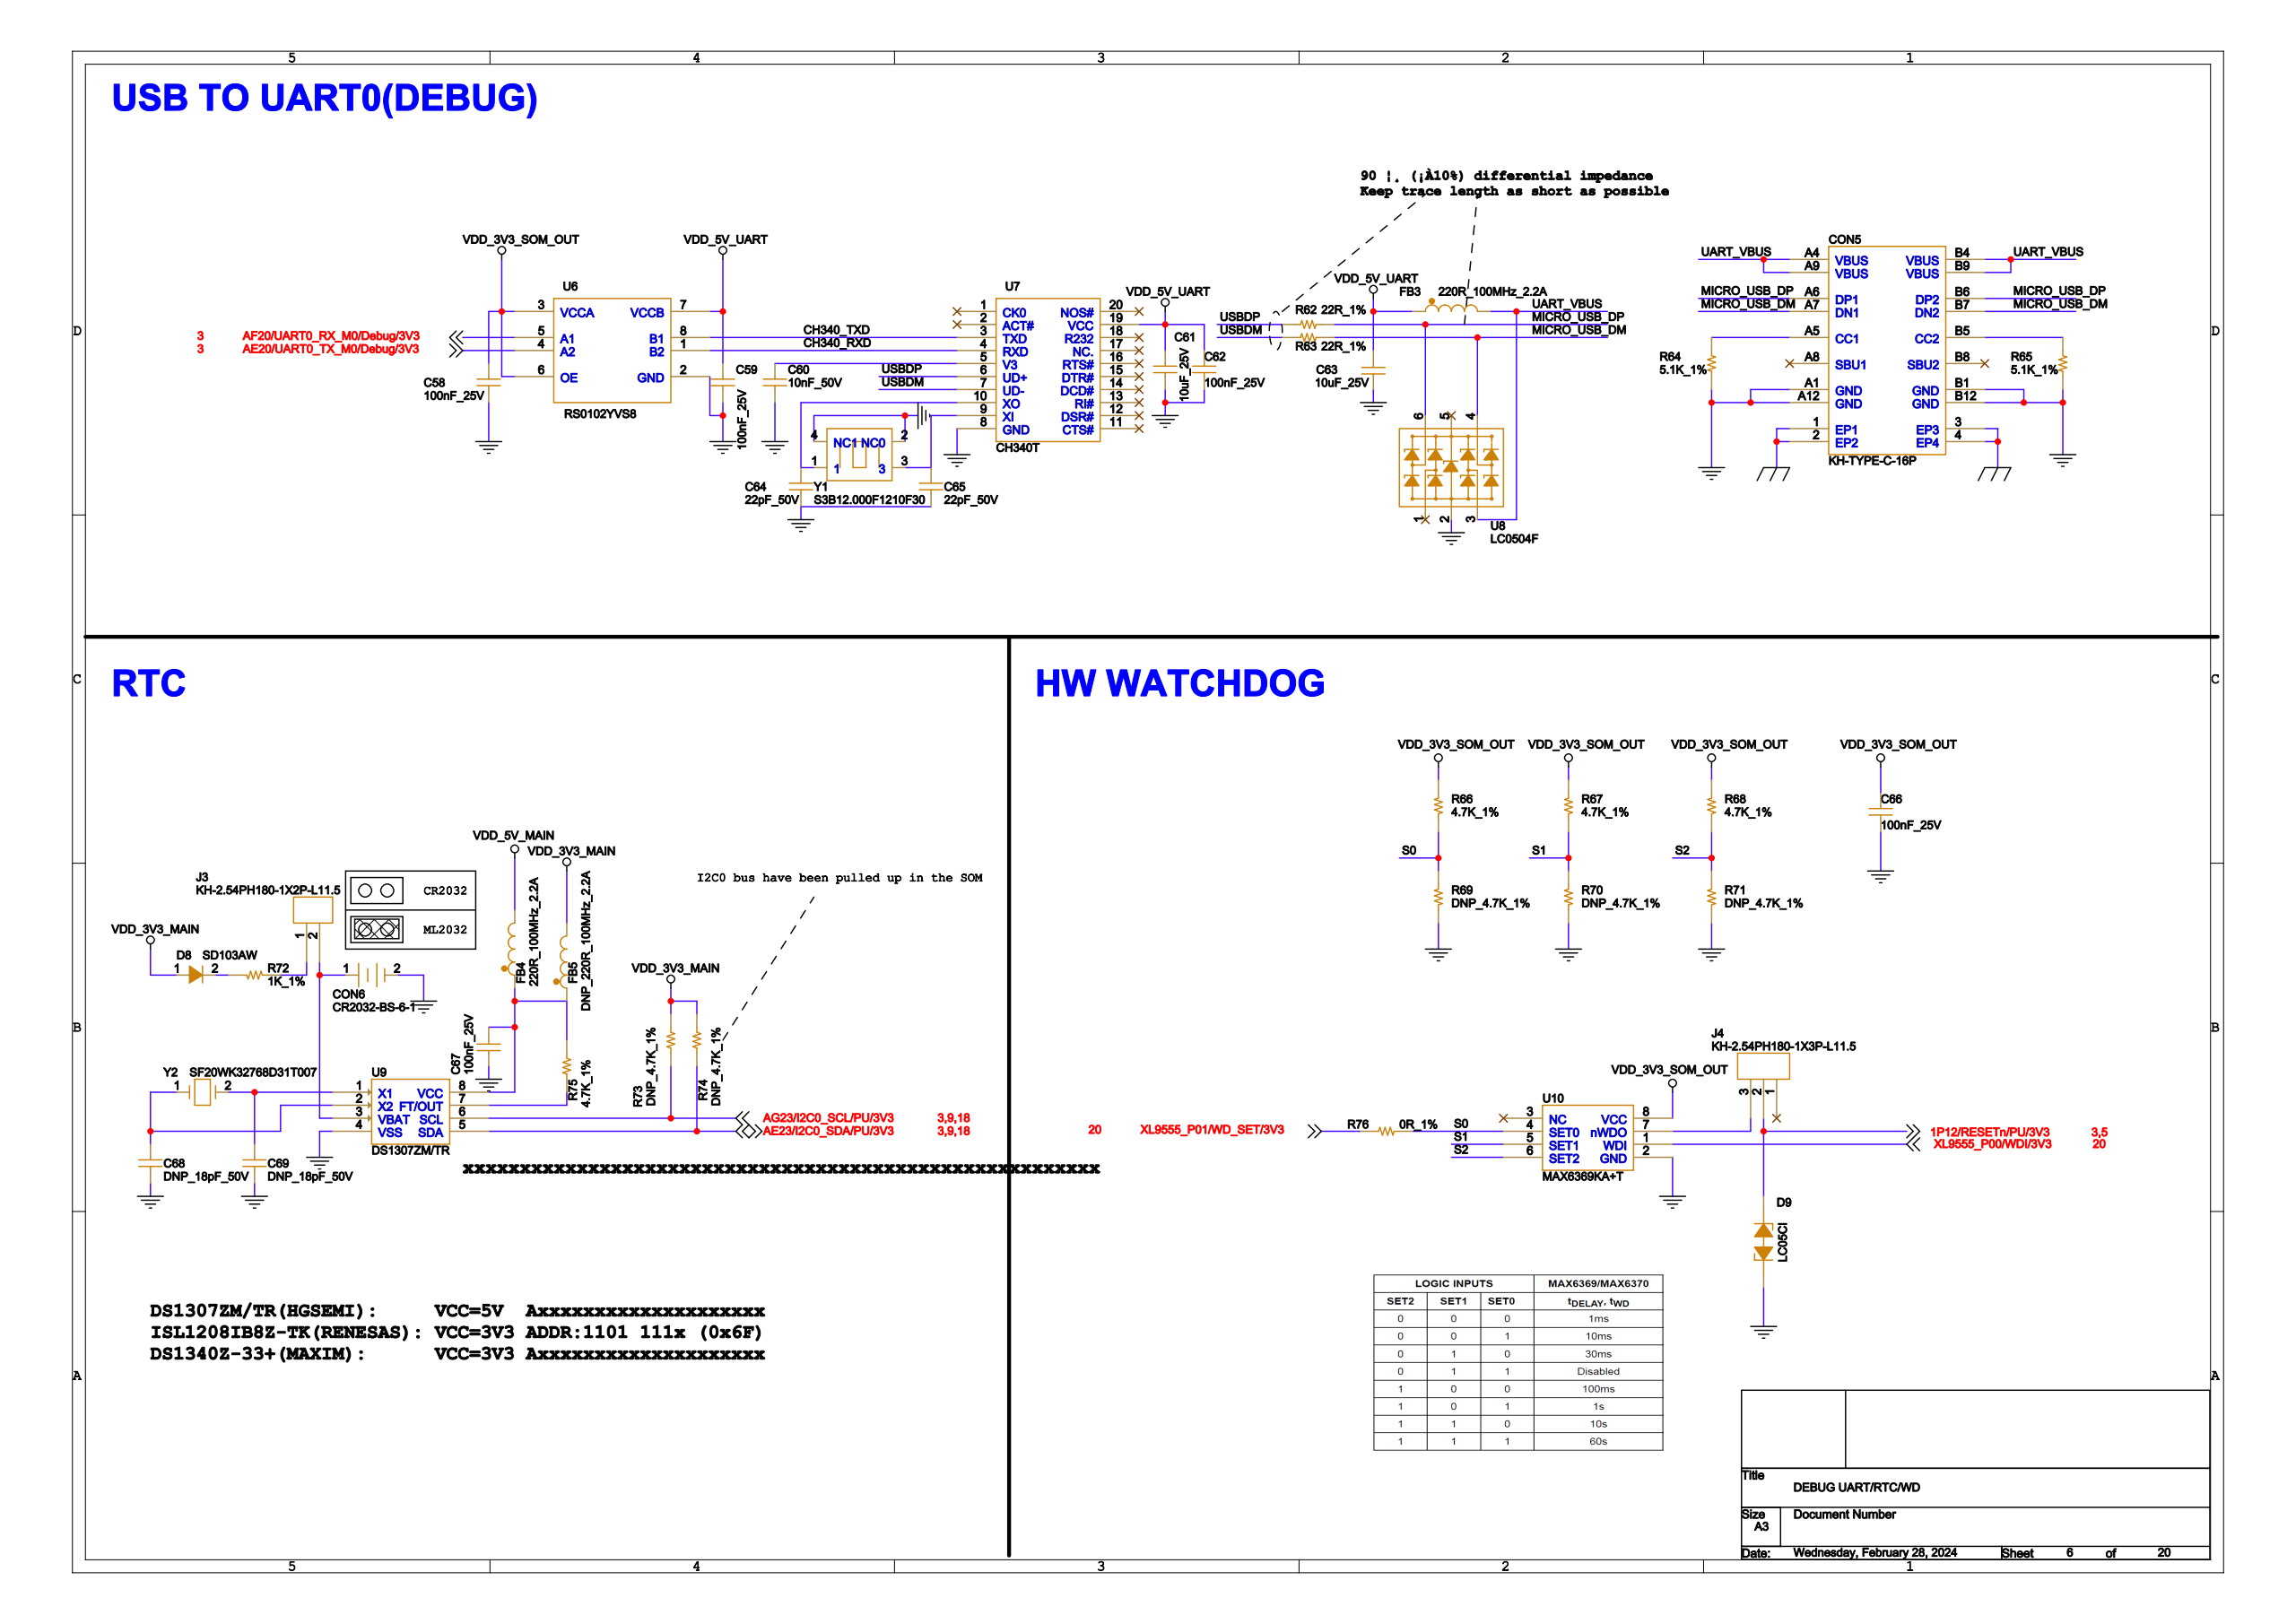Circuit board | Cadence Allegro | 1024 parts | 682 nets | one sheet of the schematic
Parts on this sheet (reference | value | footprint):
C58 | 100nF_25V | C0402
C60 | 10nF_50V | C0402
C62 | 100nF_25V | C0402
C63 | 10uF_25V | C0603
C64 | 22pF_50V | C0603
C65 | 22pF_50V | C0603
C66 | 100nF_25V | C0402
C67 | 100nF_25V | C0402
C68 | DNP_18pF_50V | C0603
C69 | DNP_18pF_50V | C0603
CON5 | KH-TYPE-C-16P | TYPE-C_16P_90_SMD
CON6 | CR2032-BS-6-1 | CON_BATTERY_CR2032
D8 | SD103AW | SOD-123_NEW
FB3 | 220R_100MHz_2A | L0603
FB4 | 220R_100MHz_2A | L0603
FB5 | DNP_220R_100MHz_2A | L0603
J3 | KH-2.54PH180-1X2P-L11.5 | HEADER_1X2P_2D54_MALE
J4 | KH-2.54PH180-1X3P-L11.5 | CON3_2D254
R62 | 22R_1% | R0402
R63 | 22R_1% | R0402
R64 | 5.1K_1% | R0402
R65 | 5.1K_1% | R0402
R66 | 4.7K_1% | R0402
R67 | 4.7K_1% | R0402
R68 | 4.7K_1% | R0402
R69 | DNP_4.7K_1% | R0402
R70 | DNP_4.7K_1% | R0402
R71 | DNP_4.7K_1% | R0402
R72 | 1K_1% | R0402
R73 | DNP_4.7K_1% | R0402
R74 | DNP_4.7K_1% | R0402
R75 | 4.7K_1% | R0402
R76 | 0R_1% | R0402
U6 | RS0102YVS8 | SOP8-20-91
U7 | CH340T | TSSOP-20
U8 | LC0504F | SOT363
U9 | DS1307ZM/TR | SOIC8_D8
U10 | MAX6369KA+T | SOT23_8
Y1 | S3B12.000F1210F30 | SMD_3225
Y2 | SF20WK32768D31T007 | SMD_2012
Nets of these parts (net: part-pin ...):
GND: C58-2 C60-2 C62-2 C63-1 C64-2 C65-2 C66-2 C67-1 C68-2 C69-2 CON5-A1 CON5-A12 CON5-B1 CON5-B12 CON6-2 R64-2 R65-2 R69-2 R70-2 R71-2 U6-2 U7-8 U8-2 U9-4 U10-2 Y1-2 Y1-4
VDD_5V_MAIN: FB4-2
EGND: CON5-1 CON5-2 CON5-3 CON5-4
1P12/RESETN/PU/3V3: J4-2
VDD_3V3_MAIN: D8-1 FB5-2 R73-1 R74-1
N21593700: C60-1 U7-5
AF20/UART0_RX_M0/DEBUG/3V3: U6-5
AE20/UART0_TX_M0/DEBUG/3V3: U6-4
AE23/I2C0_SDA/PU/3V3: R74-2 U9-5
AG23/I2C0_SCL/PU/3V3: R73-2 U9-6
VDD_3V3_SOM_OUT: C58-1 C66-1 R66-1 R67-1 R68-1 U6-3 U6-6 U10-8
N21593528: CON5-A5 R64-1
N21593482: CON5-B5 R65-1
MICRO_USB_DM: CON5-A7 CON5-B7 R63-2 U8-4
MICRO_USB_DP: CON5-A6 CON5-B6 R62-2 U8-6
UART_VBUS: CON5-A4 CON5-A9 CON5-B4 CON5-B9 FB3-2 U8-3
N21599644: J3-1 R72-1
N21599646: CON6-1 J3-2 U9-3
N21589678: J4-3 U10-7
N21599842: D8-2 R72-2
S0: R66-2 R69-1 R76-1 U10-4
S1: R67-2 R70-1 U10-5
S2: R68-2 R71-1 U10-6
N21599661: C67-2 FB4-1 FB5-1 R75-1 U9-8
N21599693: R75-2 U9-7
XL9555_P00/WDI/3V3: U10-1
XL9555_P01/WD_SET/3V3: R76-2
USBDP: R62-1 U7-6
USBDM: R63-1 U7-7
N21593733: C64-1 U7-10 Y1-1
N21593731: C65-1 U7-9 Y1-3
VDD_5V_UART: C62-1 C63-2 FB3-1 U6-7 U7-19
N21599758: C68-1 U9-2 Y2-1
N21599760: C69-1 U9-1 Y2-2
CH340_TXD: U6-8 U7-3
CH340_RXD: U6-1 U7-4